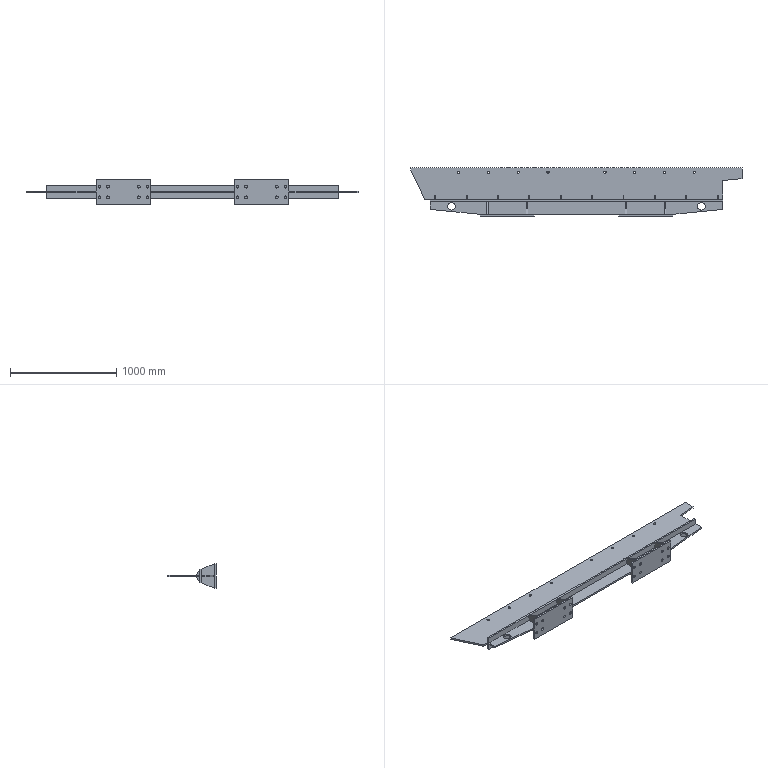Part | STEP file | Screen plate bracket (middle 1)_Default<As machined> | 32 solids | 232 faces | box 3120 x 451.736 x 230 mm | volume 29285833 mm3 | plane 180 | cylinder 52 | commonest cylinder face diameters 25 x32 21.987 x16 71.958 x4